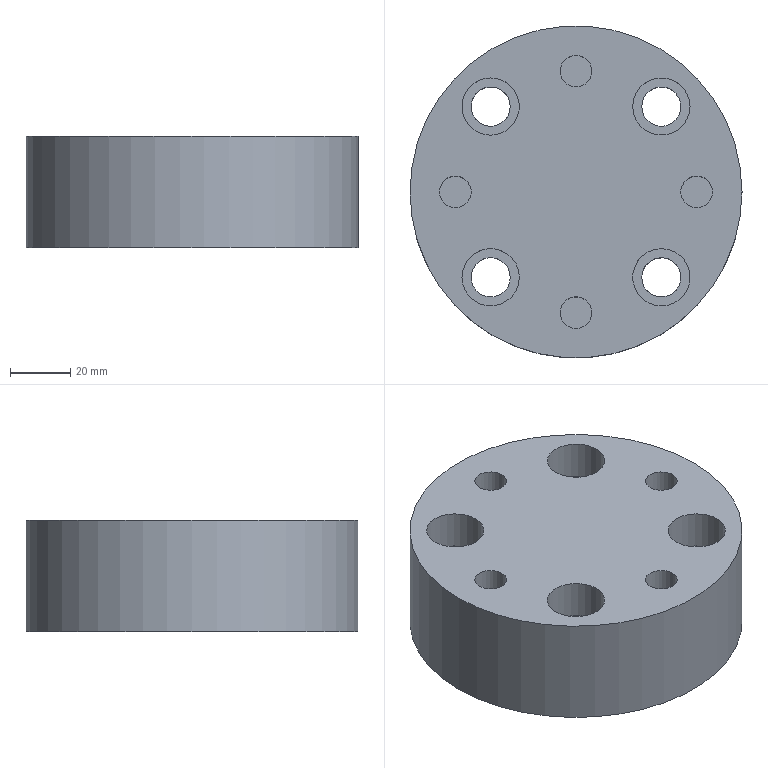Part | NX | 1 solid | 23 faces | box 110 x 110 x 37 mm | volume 315478 mm3 | cylinder 13 | plane 10 | commonest cylinder face diameters 10.5 x4 13 x4 19 x4 110 x1
STEP:
#1=CARTESIAN_POINT('',(-28.284,34.784,-37.));
#2=VERTEX_POINT('',#1);
#3=CARTESIAN_POINT('',(-28.284,28.284,-37.));
#4=DIRECTION('',(0.,0.,1.));
#5=DIRECTION('',(0.,1.,0.));
#6=AXIS2_PLACEMENT_3D('',#3,#4,#5);
#7=CIRCLE('',#6,6.5);
#8=EDGE_CURVE('',#2,#2,#7,.T.);
#9=ORIENTED_EDGE('',*,*,#8,.F.);
#10=EDGE_LOOP('',(#9));
#11=FACE_BOUND('',#10,.T.);
#12=CARTESIAN_POINT('',(-21.784,28.284,-13.));
#13=VERTEX_POINT('',#12);
#14=CARTESIAN_POINT('',(-28.284,28.284,-13.));
#15=DIRECTION('',(0.,0.,1.));
#16=DIRECTION('',(1.,0.,0.));
#17=AXIS2_PLACEMENT_3D('',#14,#15,#16);
#18=CIRCLE('',#17,6.5);
#19=EDGE_CURVE('',#13,#13,#18,.F.);
#20=ORIENTED_EDGE('',*,*,#19,.F.);
#21=EDGE_LOOP('',(#20));
#22=FACE_BOUND('',#21,.T.);
#23=CARTESIAN_POINT('',(-28.284,28.284,-37.));
#24=DIRECTION('',(0.,0.,1.));
#25=DIRECTION('',(1.,0.,0.));
#26=AXIS2_PLACEMENT_3D('',#23,#24,#25);
#27=CYLINDRICAL_SURFACE('',#26,6.5);
#28=ADVANCED_FACE('',(#11,#22),#27,.F.);
#29=CARTESIAN_POINT('',(28.284,-34.784,-37.));
#30=VERTEX_POINT('',#29);
#31=CARTESIAN_POINT('',(28.284,-28.284,-37.));
#32=DIRECTION('',(0.,0.,1.));
#33=DIRECTION('',(0.,-1.,0.));
#34=AXIS2_PLACEMENT_3D('',#31,#32,#33);
#35=CIRCLE('',#34,6.5);
#36=EDGE_CURVE('',#30,#30,#35,.T.);
#37=ORIENTED_EDGE('',*,*,#36,.F.);
#38=EDGE_LOOP('',(#37));
#39=FACE_BOUND('',#38,.T.);
#40=CARTESIAN_POINT('',(34.784,-28.284,-13.));
#41=VERTEX_POINT('',#40);
#42=CARTESIAN_POINT('',(28.284,-28.284,-13.));
#43=DIRECTION('',(0.,0.,1.));
#44=DIRECTION('',(1.,0.,0.));
#45=AXIS2_PLACEMENT_3D('',#42,#43,#44);
#46=CIRCLE('',#45,6.5);
#47=EDGE_CURVE('',#41,#41,#46,.F.);
#48=ORIENTED_EDGE('',*,*,#47,.F.);
#49=EDGE_LOOP('',(#48));
#50=FACE_BOUND('',#49,.T.);
#51=CARTESIAN_POINT('',(28.284,-28.284,-37.));
#52=DIRECTION('',(0.,0.,1.));
#53=DIRECTION('',(1.,0.,0.));
#54=AXIS2_PLACEMENT_3D('',#51,#52,#53);
#55=CYLINDRICAL_SURFACE('',#54,6.5);
#56=ADVANCED_FACE('',(#39,#50),#55,.F.);
#57=CARTESIAN_POINT('',(34.784,28.284,-37.));
#58=VERTEX_POINT('',#57);
#59=CARTESIAN_POINT('',(28.284,28.284,-37.));
#60=DIRECTION('',(0.,0.,1.));
#61=DIRECTION('',(1.,0.,0.));
#62=AXIS2_PLACEMENT_3D('',#59,#60,#61);
#63=CIRCLE('',#62,6.5);
#64=EDGE_CURVE('',#58,#58,#63,.T.);
#65=ORIENTED_EDGE('',*,*,#64,.F.);
#66=EDGE_LOOP('',(#65));
#67=FACE_BOUND('',#66,.T.);
#68=CARTESIAN_POINT('',(34.784,28.284,-13.));
#69=VERTEX_POINT('',#68);
#70=CARTESIAN_POINT('',(28.284,28.284,-13.));
#71=DIRECTION('',(0.,0.,1.));
#72=DIRECTION('',(1.,0.,0.));
#73=AXIS2_PLACEMENT_3D('',#70,#71,#72);
#74=CIRCLE('',#73,6.5);
#75=EDGE_CURVE('',#69,#69,#74,.F.);
#76=ORIENTED_EDGE('',*,*,#75,.F.);
#77=EDGE_LOOP('',(#76));
#78=FACE_BOUND('',#77,.T.);
#79=CARTESIAN_POINT('',(28.284,28.284,-37.));
#80=DIRECTION('',(0.,0.,1.));
#81=DIRECTION('',(1.,0.,0.));
#82=AXIS2_PLACEMENT_3D('',#79,#80,#81);
#83=CYLINDRICAL_SURFACE('',#82,6.5);
#84=ADVANCED_FACE('',(#67,#78),#83,.F.);
#85=CARTESIAN_POINT('',(28.284,-37.784,0.));
#86=VERTEX_POINT('',#85);
#87=CARTESIAN_POINT('',(28.284,-28.284,0.));
#88=DIRECTION('',(0.,0.,1.));
#89=DIRECTION('',(0.,-1.,0.));
#90=AXIS2_PLACEMENT_3D('',#87,#88,#89);
#91=CIRCLE('',#90,9.5);
#92=EDGE_CURVE('',#86,#86,#91,.T.);
#93=ORIENTED_EDGE('',*,*,#92,.F.);
#94=EDGE_LOOP('',(#93));
#95=FACE_BOUND('',#94,.T.);
#96=CARTESIAN_POINT('',(-28.284,37.784,0.));
#97=VERTEX_POINT('',#96);
#98=CARTESIAN_POINT('',(-28.284,28.284,0.));
#99=DIRECTION('',(0.,0.,1.));
#100=DIRECTION('',(0.,1.,0.));
#101=AXIS2_PLACEMENT_3D('',#98,#99,#100);
#102=CIRCLE('',#101,9.5);
#103=EDGE_CURVE('',#97,#97,#102,.T.);
#104=ORIENTED_EDGE('',*,*,#103,.F.);
#105=EDGE_LOOP('',(#104));
#106=FACE_BOUND('',#105,.T.);
#107=CARTESIAN_POINT('',(55.,0.,0.));
#108=VERTEX_POINT('',#107);
#109=CARTESIAN_POINT('',(0.,0.,0.));
#110=DIRECTION('',(0.,0.,1.));
#111=DIRECTION('',(1.,0.,0.));
#112=AXIS2_PLACEMENT_3D('',#109,#110,#111);
#113=CIRCLE('',#112,55.);
#114=EDGE_CURVE('',#108,#108,#113,.T.);
#115=ORIENTED_EDGE('',*,*,#114,.T.);
#116=EDGE_LOOP('',(#115));
#117=FACE_BOUND('',#116,.T.);
#118=CARTESIAN_POINT('',(-40.,5.25,0.));
#119=VERTEX_POINT('',#118);
#120=CARTESIAN_POINT('',(-40.,0.,0.));
#121=DIRECTION('',(0.,0.,1.));
#122=DIRECTION('',(0.,1.,0.));
#123=AXIS2_PLACEMENT_3D('',#120,#121,#122);
#124=CIRCLE('',#123,5.25);
#125=EDGE_CURVE('',#119,#119,#124,.T.);
#126=ORIENTED_EDGE('',*,*,#125,.F.);
#127=EDGE_LOOP('',(#126));
#128=FACE_BOUND('',#127,.T.);
#129=CARTESIAN_POINT('',(-5.25,-40.,0.));
#130=VERTEX_POINT('',#129);
#131=CARTESIAN_POINT('',(0.,-40.,0.));
#132=DIRECTION('',(0.,0.,1.));
#133=DIRECTION('',(-1.,0.,0.));
#134=AXIS2_PLACEMENT_3D('',#131,#132,#133);
#135=CIRCLE('',#134,5.25);
#136=EDGE_CURVE('',#130,#130,#135,.T.);
#137=ORIENTED_EDGE('',*,*,#136,.F.);
#138=EDGE_LOOP('',(#137));
#139=FACE_BOUND('',#138,.T.);
#140=CARTESIAN_POINT('',(5.25,40.,0.));
#141=VERTEX_POINT('',#140);
#142=CARTESIAN_POINT('',(0.,40.,0.));
#143=DIRECTION('',(0.,0.,1.));
#144=DIRECTION('',(1.,0.,0.));
#145=AXIS2_PLACEMENT_3D('',#142,#143,#144);
#146=CIRCLE('',#145,5.25);
#147=EDGE_CURVE('',#141,#141,#146,.T.);
#148=ORIENTED_EDGE('',*,*,#147,.F.);
#149=EDGE_LOOP('',(#148));
#150=FACE_BOUND('',#149,.T.);
#151=CARTESIAN_POINT('',(40.,-5.25,0.));
#152=VERTEX_POINT('',#151);
#153=CARTESIAN_POINT('',(40.,0.,0.));
#154=DIRECTION('',(0.,0.,1.));
#155=DIRECTION('',(0.,-1.,0.));
#156=AXIS2_PLACEMENT_3D('',#153,#154,#155);
#157=CIRCLE('',#156,5.25);
#158=EDGE_CURVE('',#152,#152,#157,.T.);
#159=ORIENTED_EDGE('',*,*,#158,.F.);
#160=EDGE_LOOP('',(#159));
#161=FACE_BOUND('',#160,.T.);
#162=CARTESIAN_POINT('',(37.784,28.284,0.));
#163=VERTEX_POINT('',#162);
#164=CARTESIAN_POINT('',(28.284,28.284,0.));
#165=DIRECTION('',(0.,0.,1.));
#166=DIRECTION('',(1.,0.,0.));
#167=AXIS2_PLACEMENT_3D('',#164,#165,#166);
#168=CIRCLE('',#167,9.5);
#169=EDGE_CURVE('',#163,#163,#168,.T.);
#170=ORIENTED_EDGE('',*,*,#169,.F.);
#171=EDGE_LOOP('',(#170));
#172=FACE_BOUND('',#171,.T.);
#173=CARTESIAN_POINT('',(-37.784,-28.284,0.));
#174=VERTEX_POINT('',#173);
#175=CARTESIAN_POINT('',(-28.284,-28.284,0.));
#176=DIRECTION('',(0.,0.,-1.));
#177=DIRECTION('',(-1.,0.,0.));
#178=AXIS2_PLACEMENT_3D('',#175,#176,#177);
#179=CIRCLE('',#178,9.5);
#180=EDGE_CURVE('',#174,#174,#179,.T.);
#181=ORIENTED_EDGE('',*,*,#180,.T.);
#182=EDGE_LOOP('',(#181));
#183=FACE_BOUND('',#182,.T.);
#184=CARTESIAN_POINT('',(14.142,14.142,0.));
#185=DIRECTION('',(0.,0.,1.));
#186=DIRECTION('',(1.,0.,0.));
#187=AXIS2_PLACEMENT_3D('',#184,#185,#186);
#188=PLANE('',#187);
#189=ADVANCED_FACE('',(#95,#106,#117,#128,#139,#150,#161,#172,#183),#188,.T.);
#190=CARTESIAN_POINT('',(55.,0.,-37.));
#191=VERTEX_POINT('',#190);
#192=CARTESIAN_POINT('',(0.,0.,-37.));
#193=DIRECTION('',(0.,0.,1.));
#194=DIRECTION('',(1.,0.,0.));
#195=AXIS2_PLACEMENT_3D('',#192,#193,#194);
#196=CIRCLE('',#195,55.);
#197=EDGE_CURVE('',#191,#191,#196,.T.);
#198=ORIENTED_EDGE('',*,*,#197,.T.);
#199=EDGE_LOOP('',(#198));
#200=FACE_BOUND('',#199,.T.);
#201=ORIENTED_EDGE('',*,*,#114,.F.);
#202=EDGE_LOOP('',(#201));
#203=FACE_BOUND('',#202,.T.);
#204=CARTESIAN_POINT('',(0.,0.,-37.));
#205=DIRECTION('',(0.,0.,1.));
#206=DIRECTION('',(1.,0.,0.));
#207=AXIS2_PLACEMENT_3D('',#204,#205,#206);
#208=CYLINDRICAL_SURFACE('',#207,55.);
#209=ADVANCED_FACE('',(#200,#203),#208,.T.);
#210=CARTESIAN_POINT('',(-34.784,-28.284,-13.));
#211=VERTEX_POINT('',#210);
#212=CARTESIAN_POINT('',(-28.284,-28.284,-13.));
#213=DIRECTION('',(0.,0.,-1.));
#214=DIRECTION('',(-1.,0.,0.));
#215=AXIS2_PLACEMENT_3D('',#212,#213,#214);
#216=CIRCLE('',#215,6.5);
#217=EDGE_CURVE('',#211,#211,#216,.F.);
#218=ORIENTED_EDGE('',*,*,#217,.T.);
#219=EDGE_LOOP('',(#218));
#220=FACE_BOUND('',#219,.T.);
#221=CARTESIAN_POINT('',(-34.784,-28.284,-37.));
#222=VERTEX_POINT('',#221);
#223=CARTESIAN_POINT('',(-28.284,-28.284,-37.));
#224=DIRECTION('',(0.,0.,1.));
#225=DIRECTION('',(-1.,0.,0.));
#226=AXIS2_PLACEMENT_3D('',#223,#224,#225);
#227=CIRCLE('',#226,6.5);
#228=EDGE_CURVE('',#222,#222,#227,.T.);
#229=ORIENTED_EDGE('',*,*,#228,.F.);
#230=EDGE_LOOP('',(#229));
#231=FACE_BOUND('',#230,.T.);
#232=CARTESIAN_POINT('',(-28.284,-28.284,-37.));
#233=DIRECTION('',(0.,0.,1.));
#234=DIRECTION('',(1.,0.,0.));
#235=AXIS2_PLACEMENT_3D('',#232,#233,#234);
#236=CYLINDRICAL_SURFACE('',#235,6.5);
#237=ADVANCED_FACE('',(#220,#231),#236,.F.);
#238=ORIENTED_EDGE('',*,*,#197,.F.);
#239=EDGE_LOOP('',(#238));
#240=FACE_BOUND('',#239,.T.);
#241=ORIENTED_EDGE('',*,*,#64,.T.);
#242=EDGE_LOOP('',(#241));
#243=FACE_BOUND('',#242,.T.);
#244=ORIENTED_EDGE('',*,*,#36,.T.);
#245=EDGE_LOOP('',(#244));
#246=FACE_BOUND('',#245,.T.);
#247=ORIENTED_EDGE('',*,*,#8,.T.);
#248=EDGE_LOOP('',(#247));
#249=FACE_BOUND('',#248,.T.);
#250=ORIENTED_EDGE('',*,*,#228,.T.);
#251=EDGE_LOOP('',(#250));
#252=FACE_BOUND('',#251,.T.);
#253=CARTESIAN_POINT('',(14.142,14.142,-37.));
#254=DIRECTION('',(0.,0.,1.));
#255=DIRECTION('',(1.,0.,0.));
#256=AXIS2_PLACEMENT_3D('',#253,#254,#255);
#257=PLANE('',#256);
#258=ADVANCED_FACE('',(#240,#243,#246,#249,#252),#257,.F.);
#259=CARTESIAN_POINT('',(-40.,5.25,-25.));
#260=VERTEX_POINT('',#259);
#261=CARTESIAN_POINT('',(-40.,0.,-25.));
#262=DIRECTION('',(0.,0.,1.));
#263=DIRECTION('',(0.,1.,0.));
#264=AXIS2_PLACEMENT_3D('',#261,#262,#263);
#265=CIRCLE('',#264,5.25);
#266=EDGE_CURVE('',#260,#260,#265,.F.);
#267=ORIENTED_EDGE('',*,*,#266,.T.);
#268=EDGE_LOOP('',(#267));
#269=FACE_BOUND('',#268,.T.);
#270=ORIENTED_EDGE('',*,*,#125,.T.);
#271=EDGE_LOOP('',(#270));
#272=FACE_BOUND('',#271,.T.);
#273=CARTESIAN_POINT('',(-40.,0.,-25.));
#274=DIRECTION('',(0.,0.,1.));
#275=DIRECTION('',(1.,0.,0.));
#276=AXIS2_PLACEMENT_3D('',#273,#274,#275);
#277=CYLINDRICAL_SURFACE('',#276,5.25);
#278=ADVANCED_FACE('',(#269,#272),#277,.F.);
#279=ORIENTED_EDGE('',*,*,#266,.F.);
#280=EDGE_LOOP('',(#279));
#281=FACE_BOUND('',#280,.T.);
#282=CARTESIAN_POINT('',(-40.,0.,-25.));
#283=DIRECTION('',(0.,0.,1.));
#284=DIRECTION('',(1.,0.,0.));
#285=AXIS2_PLACEMENT_3D('',#282,#283,#284);
#286=PLANE('',#285);
#287=ADVANCED_FACE('',(#281),#286,.T.);
#288=CARTESIAN_POINT('',(-5.25,-40.,-25.));
#289=VERTEX_POINT('',#288);
#290=CARTESIAN_POINT('',(0.,-40.,-25.));
#291=DIRECTION('',(0.,0.,1.));
#292=DIRECTION('',(-1.,0.,0.));
#293=AXIS2_PLACEMENT_3D('',#290,#291,#292);
#294=CIRCLE('',#293,5.25);
#295=EDGE_CURVE('',#289,#289,#294,.F.);
#296=ORIENTED_EDGE('',*,*,#295,.T.);
#297=EDGE_LOOP('',(#296));
#298=FACE_BOUND('',#297,.T.);
#299=ORIENTED_EDGE('',*,*,#136,.T.);
#300=EDGE_LOOP('',(#299));
#301=FACE_BOUND('',#300,.T.);
#302=CARTESIAN_POINT('',(0.,-40.,-25.));
#303=DIRECTION('',(0.,0.,1.));
#304=DIRECTION('',(1.,0.,0.));
#305=AXIS2_PLACEMENT_3D('',#302,#303,#304);
#306=CYLINDRICAL_SURFACE('',#305,5.25);
#307=ADVANCED_FACE('',(#298,#301),#306,.F.);
#308=ORIENTED_EDGE('',*,*,#295,.F.);
#309=EDGE_LOOP('',(#308));
#310=FACE_BOUND('',#309,.T.);
#311=CARTESIAN_POINT('',(0.,-40.,-25.));
#312=DIRECTION('',(0.,0.,1.));
#313=DIRECTION('',(1.,0.,0.));
#314=AXIS2_PLACEMENT_3D('',#311,#312,#313);
#315=PLANE('',#314);
#316=ADVANCED_FACE('',(#310),#315,.T.);
#317=CARTESIAN_POINT('',(5.25,40.,-25.));
#318=VERTEX_POINT('',#317);
#319=CARTESIAN_POINT('',(0.,40.,-25.));
#320=DIRECTION('',(0.,0.,1.));
#321=DIRECTION('',(1.,0.,0.));
#322=AXIS2_PLACEMENT_3D('',#319,#320,#321);
#323=CIRCLE('',#322,5.25);
#324=EDGE_CURVE('',#318,#318,#323,.F.);
#325=ORIENTED_EDGE('',*,*,#324,.T.);
#326=EDGE_LOOP('',(#325));
#327=FACE_BOUND('',#326,.T.);
#328=ORIENTED_EDGE('',*,*,#147,.T.);
#329=EDGE_LOOP('',(#328));
#330=FACE_BOUND('',#329,.T.);
#331=CARTESIAN_POINT('',(0.,40.,-25.));
#332=DIRECTION('',(0.,0.,1.));
#333=DIRECTION('',(1.,0.,0.));
#334=AXIS2_PLACEMENT_3D('',#331,#332,#333);
#335=CYLINDRICAL_SURFACE('',#334,5.25);
#336=ADVANCED_FACE('',(#327,#330),#335,.F.);
#337=ORIENTED_EDGE('',*,*,#324,.F.);
#338=EDGE_LOOP('',(#337));
#339=FACE_BOUND('',#338,.T.);
#340=CARTESIAN_POINT('',(0.,40.,-25.));
#341=DIRECTION('',(0.,0.,1.));
#342=DIRECTION('',(1.,0.,0.));
#343=AXIS2_PLACEMENT_3D('',#340,#341,#342);
#344=PLANE('',#343);
#345=ADVANCED_FACE('',(#339),#344,.T.);
#346=CARTESIAN_POINT('',(40.,-5.25,-25.));
#347=VERTEX_POINT('',#346);
#348=CARTESIAN_POINT('',(40.,0.,-25.));
#349=DIRECTION('',(0.,0.,1.));
#350=DIRECTION('',(0.,-1.,0.));
#351=AXIS2_PLACEMENT_3D('',#348,#349,#350);
#352=CIRCLE('',#351,5.25);
#353=EDGE_CURVE('',#347,#347,#352,.F.);
#354=ORIENTED_EDGE('',*,*,#353,.T.);
#355=EDGE_LOOP('',(#354));
#356=FACE_BOUND('',#355,.T.);
#357=ORIENTED_EDGE('',*,*,#158,.T.);
#358=EDGE_LOOP('',(#357));
#359=FACE_BOUND('',#358,.T.);
#360=CARTESIAN_POINT('',(40.,0.,-25.));
#361=DIRECTION('',(0.,0.,1.));
#362=DIRECTION('',(1.,0.,0.));
#363=AXIS2_PLACEMENT_3D('',#360,#361,#362);
#364=CYLINDRICAL_SURFACE('',#363,5.25);
#365=ADVANCED_FACE('',(#356,#359),#364,.F.);
#366=ORIENTED_EDGE('',*,*,#353,.F.);
#367=EDGE_LOOP('',(#366));
#368=FACE_BOUND('',#367,.T.);
#369=CARTESIAN_POINT('',(40.,0.,-25.));
#370=DIRECTION('',(0.,0.,1.));
#371=DIRECTION('',(1.,0.,0.));
#372=AXIS2_PLACEMENT_3D('',#369,#370,#371);
#373=PLANE('',#372);
#374=ADVANCED_FACE('',(#368),#373,.T.);
#375=CARTESIAN_POINT('',(37.784,28.284,-13.));
#376=VERTEX_POINT('',#375);
#377=CARTESIAN_POINT('',(28.284,28.284,-13.));
#378=DIRECTION('',(0.,0.,1.));
#379=DIRECTION('',(1.,0.,0.));
#380=AXIS2_PLACEMENT_3D('',#377,#378,#379);
#381=CIRCLE('',#380,9.5);
#382=EDGE_CURVE('',#376,#376,#381,.F.);
#383=ORIENTED_EDGE('',*,*,#382,.F.);
#384=EDGE_LOOP('',(#383));
#385=FACE_BOUND('',#384,.T.);
#386=ORIENTED_EDGE('',*,*,#75,.T.);
#387=EDGE_LOOP('',(#386));
#388=FACE_BOUND('',#387,.T.);
#389=CARTESIAN_POINT('',(28.284,28.284,-13.));
#390=DIRECTION('',(0.,0.,1.));
#391=DIRECTION('',(1.,0.,0.));
#392=AXIS2_PLACEMENT_3D('',#389,#390,#391);
#393=PLANE('',#392);
#394=ADVANCED_FACE('',(#385,#388),#393,.T.);
#395=ORIENTED_EDGE('',*,*,#382,.T.);
#396=EDGE_LOOP('',(#395));
#397=FACE_BOUND('',#396,.T.);
#398=ORIENTED_EDGE('',*,*,#169,.T.);
#399=EDGE_LOOP('',(#398));
#400=FACE_BOUND('',#399,.T.);
#401=CARTESIAN_POINT('',(28.284,28.284,-13.));
#402=DIRECTION('',(0.,0.,1.));
#403=DIRECTION('',(1.,0.,0.));
#404=AXIS2_PLACEMENT_3D('',#401,#402,#403);
#405=CYLINDRICAL_SURFACE('',#404,9.5);
#406=ADVANCED_FACE('',(#397,#400),#405,.F.);
#407=CARTESIAN_POINT('',(-37.784,-28.284,-13.));
#408=VERTEX_POINT('',#407);
#409=CARTESIAN_POINT('',(-28.284,-28.284,-13.));
#410=DIRECTION('',(0.,0.,-1.));
#411=DIRECTION('',(-1.,0.,0.));
#412=AXIS2_PLACEMENT_3D('',#409,#410,#411);
#413=CIRCLE('',#412,9.5);
#414=EDGE_CURVE('',#408,#408,#413,.F.);
#415=ORIENTED_EDGE('',*,*,#414,.T.);
#416=EDGE_LOOP('',(#415));
#417=FACE_BOUND('',#416,.T.);
#418=ORIENTED_EDGE('',*,*,#217,.F.);
#419=EDGE_LOOP('',(#418));
#420=FACE_BOUND('',#419,.T.);
#421=CARTESIAN_POINT('',(-28.284,-28.284,-13.));
#422=DIRECTION('',(0.,0.,-1.));
#423=DIRECTION('',(-1.,0.,0.));
#424=AXIS2_PLACEMENT_3D('',#421,#422,#423);
#425=PLANE('',#424);
#426=ADVANCED_FACE('',(#417,#420),#425,.F.);
#427=ORIENTED_EDGE('',*,*,#414,.F.);
#428=EDGE_LOOP('',(#427));
#429=FACE_BOUND('',#428,.T.);
#430=ORIENTED_EDGE('',*,*,#180,.F.);
#431=EDGE_LOOP('',(#430));
#432=FACE_BOUND('',#431,.T.);
#433=CARTESIAN_POINT('',(-28.284,-28.284,-13.));
#434=DIRECTION('',(0.,0.,1.));
#435=DIRECTION('',(1.,0.,0.));
#436=AXIS2_PLACEMENT_3D('',#433,#434,#435);
#437=CYLINDRICAL_SURFACE('',#436,9.5);
#438=ADVANCED_FACE('',(#429,#432),#437,.F.);
#439=CARTESIAN_POINT('',(-28.284,37.784,-13.));
#440=VERTEX_POINT('',#439);
#441=CARTESIAN_POINT('',(-28.284,28.284,-13.));
#442=DIRECTION('',(0.,0.,1.));
#443=DIRECTION('',(0.,1.,0.));
#444=AXIS2_PLACEMENT_3D('',#441,#442,#443);
#445=CIRCLE('',#444,9.5);
#446=EDGE_CURVE('',#440,#440,#445,.F.);
#447=ORIENTED_EDGE('',*,*,#446,.F.);
#448=EDGE_LOOP('',(#447));
#449=FACE_BOUND('',#448,.T.);
#450=ORIENTED_EDGE('',*,*,#19,.T.);
#451=EDGE_LOOP('',(#450));
#452=FACE_BOUND('',#451,.T.);
#453=CARTESIAN_POINT('',(-28.284,28.284,-13.));
#454=DIRECTION('',(0.,0.,1.));
#455=DIRECTION('',(1.,0.,0.));
#456=AXIS2_PLACEMENT_3D('',#453,#454,#455);
#457=PLANE('',#456);
#458=ADVANCED_FACE('',(#449,#452),#457,.T.);
#459=ORIENTED_EDGE('',*,*,#446,.T.);
#460=EDGE_LOOP('',(#459));
#461=FACE_BOUND('',#460,.T.);
#462=ORIENTED_EDGE('',*,*,#103,.T.);
#463=EDGE_LOOP('',(#462));
#464=FACE_BOUND('',#463,.T.);
#465=CARTESIAN_POINT('',(-28.284,28.284,-13.));
#466=DIRECTION('',(0.,0.,1.));
#467=DIRECTION('',(1.,0.,0.));
#468=AXIS2_PLACEMENT_3D('',#465,#466,#467);
#469=CYLINDRICAL_SURFACE('',#468,9.5);
#470=ADVANCED_FACE('',(#461,#464),#469,.F.);
#471=CARTESIAN_POINT('',(28.284,-37.784,-13.));
#472=VERTEX_POINT('',#471);
#473=CARTESIAN_POINT('',(28.284,-28.284,-13.));
#474=DIRECTION('',(0.,0.,1.));
#475=DIRECTION('',(0.,-1.,0.));
#476=AXIS2_PLACEMENT_3D('',#473,#474,#475);
#477=CIRCLE('',#476,9.5);
#478=EDGE_CURVE('',#472,#472,#477,.F.);
#479=ORIENTED_EDGE('',*,*,#478,.F.);
#480=EDGE_LOOP('',(#479));
#481=FACE_BOUND('',#480,.T.);
#482=ORIENTED_EDGE('',*,*,#47,.T.);
#483=EDGE_LOOP('',(#482));
#484=FACE_BOUND('',#483,.T.);
#485=CARTESIAN_POINT('',(28.284,-28.284,-13.));
#486=DIRECTION('',(0.,0.,1.));
#487=DIRECTION('',(1.,0.,0.));
#488=AXIS2_PLACEMENT_3D('',#485,#486,#487);
#489=PLANE('',#488);
#490=ADVANCED_FACE('',(#481,#484),#489,.T.);
#491=ORIENTED_EDGE('',*,*,#478,.T.);
#492=EDGE_LOOP('',(#491));
#493=FACE_BOUND('',#492,.T.);
#494=ORIENTED_EDGE('',*,*,#92,.T.);
#495=EDGE_LOOP('',(#494));
#496=FACE_BOUND('',#495,.T.);
#497=CARTESIAN_POINT('',(28.284,-28.284,-13.));
#498=DIRECTION('',(0.,0.,1.));
#499=DIRECTION('',(1.,0.,0.));
#500=AXIS2_PLACEMENT_3D('',#497,#498,#499);
#501=CYLINDRICAL_SURFACE('',#500,9.5);
#502=ADVANCED_FACE('',(#493,#496),#501,.F.);
#503=CLOSED_SHELL('',(#28,#56,#84,#189,#209,#237,#258,#278,#287,#307,#316,#336,#345,#365,#374,#394,#406,#426,#438,#458,#470,#490,#502));
#504=MANIFOLD_SOLID_BREP('',#503);
#505=(LENGTH_UNIT()NAMED_UNIT(*)SI_UNIT(.MILLI.,.METRE.));
#506=UNCERTAINTY_MEASURE_WITH_UNIT(LENGTH_MEASURE(0.00001),#505,'','');
#507=(NAMED_UNIT(*)PLANE_ANGLE_UNIT()SI_UNIT($,.RADIAN.));
#508=(NAMED_UNIT(*)SI_UNIT($,.STERADIAN.)SOLID_ANGLE_UNIT());
#509=(GEOMETRIC_REPRESENTATION_CONTEXT(3)GLOBAL_UNCERTAINTY_ASSIGNED_CONTEXT((#506))GLOBAL_UNIT_ASSIGNED_CONTEXT((#505,#507,#508))REPRESENTATION_CONTEXT('',''));
#510=ADVANCED_BREP_SHAPE_REPRESENTATION('',(#504),#509);